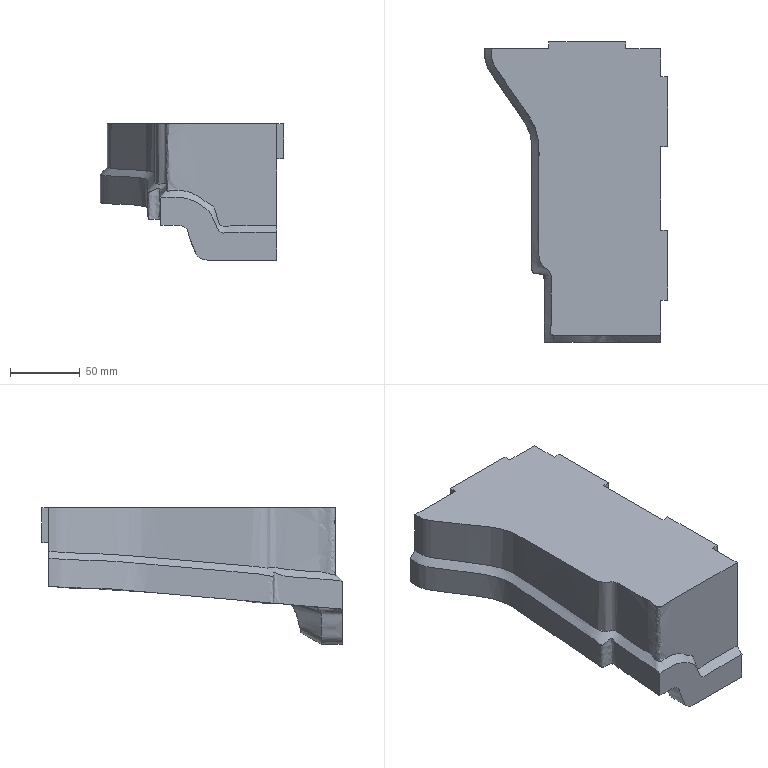Part | NX | features solid 2 | 1 solid | 37 faces | box 131.066 x 215 x 97.901 mm | volume 869941 mm3 | plane 25 | spline 7 | cylinder 5 | commonest cylinder face diameters 30 x5